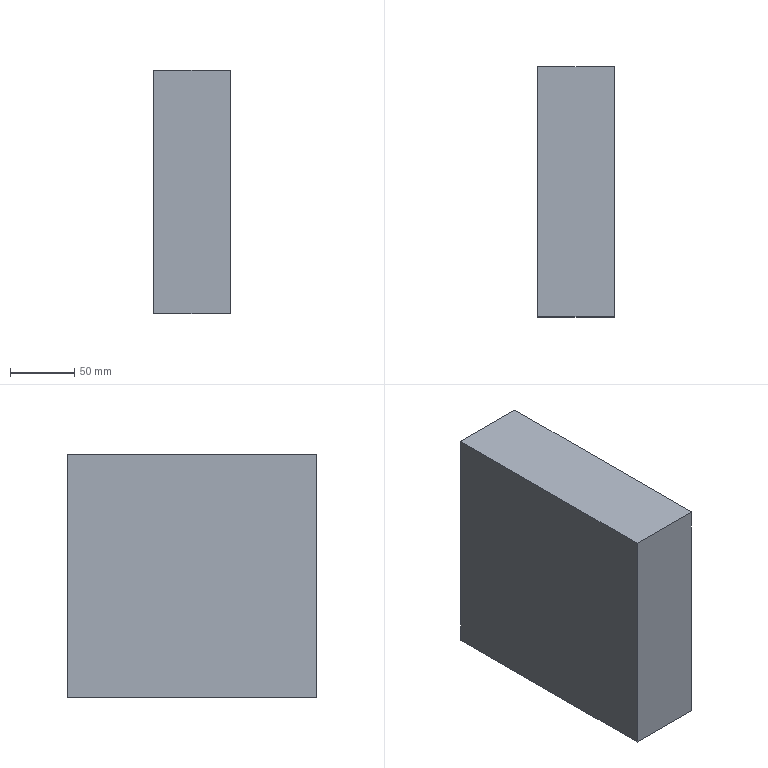Part | STEP file | lll_id4186_x_t | 1 solid | 10 faces | box 60 x 195 x 190 mm | volume 2201737 mm3 | plane 6 | cylinder 2 | cone 2 | commonest cylinder face diameters 17.506 x2
STEP:
#1=CARTESIAN_POINT('',(2356.188,-450.,-370.));
#2=VERTEX_POINT('',#1);
#3=CARTESIAN_POINT('',(2347.435,-450.,-370.));
#4=DIRECTION('',(0.,0.,1.));
#5=DIRECTION('',(1.,0.,0.));
#6=AXIS2_PLACEMENT_3D('',#3,#4,#5);
#7=CIRCLE('',#6,8.753);
#8=EDGE_CURVE('',#2,#2,#7,.T.);
#9=ORIENTED_EDGE('',*,*,#8,.T.);
#10=EDGE_LOOP('',(#9));
#11=FACE_BOUND('',#10,.T.);
#12=CARTESIAN_POINT('',(2317.435,-405.,-370.));
#13=VERTEX_POINT('',#12);
#14=CARTESIAN_POINT('',(2377.435,-405.,-370.));
#15=VERTEX_POINT('',#14);
#16=CARTESIAN_POINT('',(4563.751,-405.,-370.));
#17=DIRECTION('',(1.,0.,0.));
#18=VECTOR('',#17,1.);
#19=LINE('',#16,#18);
#20=EDGE_CURVE('',#13,#15,#19,.T.);
#21=ORIENTED_EDGE('',*,*,#20,.T.);
#22=CARTESIAN_POINT('',(2377.435,-600.,-370.));
#23=VERTEX_POINT('',#22);
#24=CARTESIAN_POINT('',(2377.435,-600.,-370.));
#25=DIRECTION('',(0.,1.,0.));
#26=VECTOR('',#25,1.);
#27=LINE('',#24,#26);
#28=EDGE_CURVE('',#23,#15,#27,.T.);
#29=ORIENTED_EDGE('',*,*,#28,.F.);
#30=CARTESIAN_POINT('',(2317.435,-600.,-370.));
#31=VERTEX_POINT('',#30);
#32=CARTESIAN_POINT('',(2132.435,-600.,-370.));
#33=DIRECTION('',(1.,0.,0.));
#34=VECTOR('',#33,1.);
#35=LINE('',#32,#34);
#36=EDGE_CURVE('',#31,#23,#35,.T.);
#37=ORIENTED_EDGE('',*,*,#36,.F.);
#38=CARTESIAN_POINT('',(2317.435,-1.,-370.));
#39=DIRECTION('',(0.,1.,0.));
#40=VECTOR('',#39,1.);
#41=LINE('',#38,#40);
#42=EDGE_CURVE('',#31,#13,#41,.T.);
#43=ORIENTED_EDGE('',*,*,#42,.T.);
#44=EDGE_LOOP('',(#21,#29,#37,#43));
#45=FACE_BOUND('',#44,.T.);
#46=CARTESIAN_POINT('',(2356.188,-550.,-370.));
#47=VERTEX_POINT('',#46);
#48=CARTESIAN_POINT('',(2347.435,-550.,-370.));
#49=DIRECTION('',(0.,0.,1.));
#50=DIRECTION('',(1.,0.,0.));
#51=AXIS2_PLACEMENT_3D('',#48,#49,#50);
#52=CIRCLE('',#51,8.753);
#53=EDGE_CURVE('',#47,#47,#52,.T.);
#54=ORIENTED_EDGE('',*,*,#53,.T.);
#55=EDGE_LOOP('',(#54));
#56=FACE_BOUND('',#55,.T.);
#57=CARTESIAN_POINT('',(4563.751,-1.,-370.));
#58=DIRECTION('',(0.,0.,-1.));
#59=DIRECTION('',(-1.,0.,0.));
#60=AXIS2_PLACEMENT_3D('',#57,#58,#59);
#61=PLANE('',#60);
#62=ADVANCED_FACE('',(#11,#45,#56),#61,.T.);
#63=CARTESIAN_POINT('',(2317.435,-600.,-180.));
#64=VERTEX_POINT('',#63);
#65=CARTESIAN_POINT('',(2317.435,-600.,-160.));
#66=DIRECTION('',(0.,0.,1.));
#67=VECTOR('',#66,1.);
#68=LINE('',#65,#67);
#69=EDGE_CURVE('',#31,#64,#68,.T.);
#70=ORIENTED_EDGE('',*,*,#69,.F.);
#71=ORIENTED_EDGE('',*,*,#36,.T.);
#72=CARTESIAN_POINT('',(2377.435,-600.,-180.));
#73=VERTEX_POINT('',#72);
#74=CARTESIAN_POINT('',(2377.435,-600.,-182.5));
#75=DIRECTION('',(0.,0.,-1.));
#76=VECTOR('',#75,1.);
#77=LINE('',#74,#76);
#78=EDGE_CURVE('',#73,#23,#77,.T.);
#79=ORIENTED_EDGE('',*,*,#78,.F.);
#80=CARTESIAN_POINT('',(2132.435,-600.,-180.));
#81=DIRECTION('',(1.,0.,0.));
#82=VECTOR('',#81,1.);
#83=LINE('',#80,#82);
#84=EDGE_CURVE('',#64,#73,#83,.T.);
#85=ORIENTED_EDGE('',*,*,#84,.F.);
#86=EDGE_LOOP('',(#70,#71,#79,#85));
#87=FACE_OUTER_BOUND('',#86,.T.);
#88=CARTESIAN_POINT('',(2132.435,-600.,-160.));
#89=DIRECTION('',(0.,-1.,0.));
#90=DIRECTION('',(0.,0.,-1.));
#91=AXIS2_PLACEMENT_3D('',#88,#89,#90);
#92=PLANE('',#91);
#93=ADVANCED_FACE('',(#87),#92,.T.);
#94=ORIENTED_EDGE('',*,*,#42,.F.);
#95=ORIENTED_EDGE('',*,*,#69,.T.);
#96=CARTESIAN_POINT('',(2317.435,-405.,-180.));
#97=VERTEX_POINT('',#96);
#98=CARTESIAN_POINT('',(2317.435,0.,-180.));
#99=DIRECTION('',(0.,-1.,0.));
#100=VECTOR('',#99,1.);
#101=LINE('',#98,#100);
#102=EDGE_CURVE('',#97,#64,#101,.T.);
#103=ORIENTED_EDGE('',*,*,#102,.F.);
#104=CARTESIAN_POINT('',(2317.435,-405.,-251.25));
#105=DIRECTION('',(0.,0.,-1.));
#106=VECTOR('',#105,1.);
#107=LINE('',#104,#106);
#108=EDGE_CURVE('',#97,#13,#107,.T.);
#109=ORIENTED_EDGE('',*,*,#108,.T.);
#110=EDGE_LOOP('',(#94,#95,#103,#109));
#111=FACE_OUTER_BOUND('',#110,.T.);
#112=CARTESIAN_POINT('',(2317.435,0.,-251.25));
#113=DIRECTION('',(1.,0.,0.));
#114=DIRECTION('',(0.,0.,-1.));
#115=AXIS2_PLACEMENT_3D('',#112,#113,#114);
#116=PLANE('',#115);
#117=ADVANCED_FACE('',(#111),#116,.F.);
#118=ORIENTED_EDGE('',*,*,#102,.T.);
#119=ORIENTED_EDGE('',*,*,#84,.T.);
#120=CARTESIAN_POINT('',(2377.435,-405.,-180.));
#121=VERTEX_POINT('',#120);
#122=CARTESIAN_POINT('',(2377.435,-1.,-180.));
#123=DIRECTION('',(0.,1.,0.));
#124=VECTOR('',#123,1.);
#125=LINE('',#122,#124);
#126=EDGE_CURVE('',#73,#121,#125,.T.);
#127=ORIENTED_EDGE('',*,*,#126,.T.);
#128=CARTESIAN_POINT('',(4563.751,-405.,-180.));
#129=DIRECTION('',(1.,0.,0.));
#130=VECTOR('',#129,1.);
#131=LINE('',#128,#130);
#132=EDGE_CURVE('',#97,#121,#131,.T.);
#133=ORIENTED_EDGE('',*,*,#132,.F.);
#134=EDGE_LOOP('',(#118,#119,#127,#133));
#135=FACE_OUTER_BOUND('',#134,.T.);
#136=CARTESIAN_POINT('',(4563.751,-1.,-180.));
#137=DIRECTION('',(0.,0.,-1.));
#138=DIRECTION('',(-1.,0.,0.));
#139=AXIS2_PLACEMENT_3D('',#136,#137,#138);
#140=PLANE('',#139);
#141=ADVANCED_FACE('',(#135),#140,.F.);
#142=CARTESIAN_POINT('',(2377.435,-405.,-182.5));
#143=DIRECTION('',(0.,0.,-1.));
#144=VECTOR('',#143,1.);
#145=LINE('',#142,#144);
#146=EDGE_CURVE('',#121,#15,#145,.T.);
#147=ORIENTED_EDGE('',*,*,#146,.F.);
#148=ORIENTED_EDGE('',*,*,#126,.F.);
#149=ORIENTED_EDGE('',*,*,#78,.T.);
#150=ORIENTED_EDGE('',*,*,#28,.T.);
#151=EDGE_LOOP('',(#147,#148,#149,#150));
#152=FACE_OUTER_BOUND('',#151,.T.);
#153=CARTESIAN_POINT('',(2377.435,-600.,-182.5));
#154=DIRECTION('',(1.,0.,0.));
#155=DIRECTION('',(0.,0.,-1.));
#156=AXIS2_PLACEMENT_3D('',#153,#154,#155);
#157=PLANE('',#156);
#158=ADVANCED_FACE('',(#152),#157,.T.);
#159=ORIENTED_EDGE('',*,*,#146,.T.);
#160=ORIENTED_EDGE('',*,*,#20,.F.);
#161=ORIENTED_EDGE('',*,*,#108,.F.);
#162=ORIENTED_EDGE('',*,*,#132,.T.);
#163=EDGE_LOOP('',(#159,#160,#161,#162));
#164=FACE_OUTER_BOUND('',#163,.T.);
#165=CARTESIAN_POINT('',(2347.435,-405.,-250.));
#166=DIRECTION('',(0.,-1.,0.));
#167=DIRECTION('',(0.,0.,1.));
#168=AXIS2_PLACEMENT_3D('',#165,#166,#167);
#169=PLANE('',#168);
#170=ADVANCED_FACE('',(#164),#169,.F.);
#171=CARTESIAN_POINT('',(2356.188,-450.,-328.747));
#172=VERTEX_POINT('',#171);
#173=CARTESIAN_POINT('',(2347.435,-450.,-328.747));
#174=DIRECTION('',(0.,0.,1.));
#175=DIRECTION('',(1.,0.,0.));
#176=AXIS2_PLACEMENT_3D('',#173,#174,#175);
#177=CIRCLE('',#176,8.753);
#178=EDGE_CURVE('',#172,#172,#177,.T.);
#179=ORIENTED_EDGE('',*,*,#178,.T.);
#180=EDGE_LOOP('',(#179));
#181=FACE_BOUND('',#180,.T.);
#182=ORIENTED_EDGE('',*,*,#8,.F.);
#183=EDGE_LOOP('',(#182));
#184=FACE_BOUND('',#183,.T.);
#185=CARTESIAN_POINT('',(2347.435,-450.,-370.));
#186=DIRECTION('',(0.,0.,1.));
#187=DIRECTION('',(-1.,0.,0.));
#188=AXIS2_PLACEMENT_3D('',#185,#186,#187);
#189=CYLINDRICAL_SURFACE('',#188,8.753);
#190=ADVANCED_FACE('',(#181,#184),#189,.F.);
#191=CARTESIAN_POINT('',(2347.435,-450.,-319.994));
#192=VERTEX_POINT('',#191);
#193=VERTEX_LOOP('',#192);
#194=FACE_BOUND('',#193,.T.);
#195=ORIENTED_EDGE('',*,*,#178,.F.);
#196=EDGE_LOOP('',(#195));
#197=FACE_BOUND('',#196,.T.);
#198=CARTESIAN_POINT('',(2347.435,-450.,-328.747));
#199=DIRECTION('',(0.,0.,-1.));
#200=DIRECTION('',(1.,0.,0.));
#201=AXIS2_PLACEMENT_3D('',#198,#199,#200);
#202=CONICAL_SURFACE('',#201,8.753,45.);
#203=ADVANCED_FACE('',(#194,#197),#202,.F.);
#204=CARTESIAN_POINT('',(2356.188,-550.,-328.747));
#205=VERTEX_POINT('',#204);
#206=CARTESIAN_POINT('',(2347.435,-550.,-328.747));
#207=DIRECTION('',(0.,0.,1.));
#208=DIRECTION('',(1.,0.,0.));
#209=AXIS2_PLACEMENT_3D('',#206,#207,#208);
#210=CIRCLE('',#209,8.753);
#211=EDGE_CURVE('',#205,#205,#210,.T.);
#212=ORIENTED_EDGE('',*,*,#211,.T.);
#213=EDGE_LOOP('',(#212));
#214=FACE_BOUND('',#213,.T.);
#215=ORIENTED_EDGE('',*,*,#53,.F.);
#216=EDGE_LOOP('',(#215));
#217=FACE_BOUND('',#216,.T.);
#218=CARTESIAN_POINT('',(2347.435,-550.,-370.));
#219=DIRECTION('',(0.,0.,1.));
#220=DIRECTION('',(-1.,0.,0.));
#221=AXIS2_PLACEMENT_3D('',#218,#219,#220);
#222=CYLINDRICAL_SURFACE('',#221,8.753);
#223=ADVANCED_FACE('',(#214,#217),#222,.F.);
#224=CARTESIAN_POINT('',(2347.435,-550.,-319.994));
#225=VERTEX_POINT('',#224);
#226=VERTEX_LOOP('',#225);
#227=FACE_BOUND('',#226,.T.);
#228=ORIENTED_EDGE('',*,*,#211,.F.);
#229=EDGE_LOOP('',(#228));
#230=FACE_BOUND('',#229,.T.);
#231=CARTESIAN_POINT('',(2347.435,-550.,-328.747));
#232=DIRECTION('',(0.,0.,-1.));
#233=DIRECTION('',(1.,0.,0.));
#234=AXIS2_PLACEMENT_3D('',#231,#232,#233);
#235=CONICAL_SURFACE('',#234,8.753,45.);
#236=ADVANCED_FACE('',(#227,#230),#235,.F.);
#237=CLOSED_SHELL('',(#62,#93,#117,#141,#158,#170,#190,#203,#223,#236));
#238=MANIFOLD_SOLID_BREP('',#237);
#239=(LENGTH_UNIT()NAMED_UNIT(*)SI_UNIT(.MILLI.,.METRE.));
#240=UNCERTAINTY_MEASURE_WITH_UNIT(LENGTH_MEASURE(0.00002),#239,'','');
#241=(NAMED_UNIT(*)PLANE_ANGLE_UNIT()SI_UNIT($,.RADIAN.));
#242=PLANE_ANGLE_MEASURE_WITH_UNIT(PLANE_ANGLE_MEASURE(0.01745),#241);
#243=DIMENSIONAL_EXPONENTS(0.,0.,0.,0.,0.,0.,0.);
#244=(CONVERSION_BASED_UNIT('DEGREE',#242)NAMED_UNIT(#243)PLANE_ANGLE_UNIT());
#245=(NAMED_UNIT(*)SI_UNIT($,.STERADIAN.)SOLID_ANGLE_UNIT());
#246=(GEOMETRIC_REPRESENTATION_CONTEXT(3)GLOBAL_UNCERTAINTY_ASSIGNED_CONTEXT((#240))GLOBAL_UNIT_ASSIGNED_CONTEXT((#239,#244,#245))REPRESENTATION_CONTEXT('',''));
#247=ADVANCED_BREP_SHAPE_REPRESENTATION('',(#238),#246);